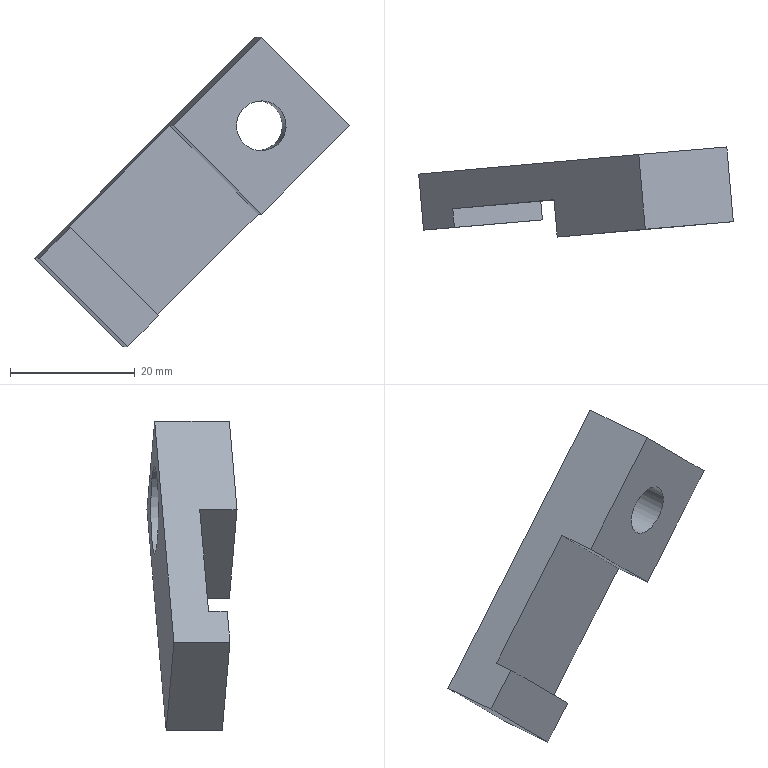Part | NX | features solid 2 | 1 solid | 13 faces | box 50.355 x 14.419 x 49.497 mm | volume 7701 mm3 | plane 11 | cylinder 1 | spline 1 | commonest cylinder face diameters 14 x1
STEP:
#1=CARTESIAN_POINT('',(-431.743,30.487,53.445));
#2=VERTEX_POINT('',#1);
#3=CARTESIAN_POINT('',(-415.541,31.905,69.708));
#4=VERTEX_POINT('',#3);
#5=CARTESIAN_POINT('',(-431.743,30.487,53.445));
#6=DIRECTION('',(0.7044,0.06163,0.7071));
#7=VECTOR('',#6,1000.);
#8=LINE('',#5,#7);
#9=EDGE_CURVE('',#2,#4,#8,.T.);
#10=ORIENTED_EDGE('',*,*,#9,.T.);
#11=CARTESIAN_POINT('',(-429.629,30.672,83.85));
#12=VERTEX_POINT('',#11);
#13=CARTESIAN_POINT('',(-415.541,31.905,69.708));
#14=DIRECTION('',(-0.7044,-0.06163,0.7071));
#15=VECTOR('',#14,1000.);
#16=LINE('',#13,#15);
#17=EDGE_CURVE('',#4,#12,#16,.T.);
#18=ORIENTED_EDGE('',*,*,#17,.T.);
#19=CARTESIAN_POINT('',(-445.831,29.255,67.587));
#20=VERTEX_POINT('',#19);
#21=CARTESIAN_POINT('',(-445.831,29.255,67.587));
#22=DIRECTION('',(0.7044,0.06163,0.7071));
#23=VECTOR('',#22,1000.);
#24=LINE('',#21,#23);
#25=EDGE_CURVE('',#20,#12,#24,.T.);
#26=ORIENTED_EDGE('',*,*,#25,.F.);
#27=CARTESIAN_POINT('',(-445.831,29.255,67.587));
#28=DIRECTION('',(0.7044,0.06163,-0.7071));
#29=VECTOR('',#28,1000.);
#30=LINE('',#27,#29);
#31=EDGE_CURVE('',#20,#2,#30,.T.);
#32=ORIENTED_EDGE('',*,*,#31,.T.);
#33=EDGE_LOOP('',(#10,#18,#26,#32));
#34=FACE_BOUND('',#33,.T.);
#35=CARTESIAN_POINT('',(-445.831,29.255,67.587));
#36=DIRECTION('',(-0.08716,0.9962,0.));
#37=DIRECTION('',(0.421,0.03683,0.9063));
#38=AXIS2_PLACEMENT_3D('',#35,#36,#37);
#39=PLANE('',#38);
#40=ADVANCED_FACE('',(#34),#39,.F.);
#41=CARTESIAN_POINT('',(-419.24,32.585,85.541));
#42=VERTEX_POINT('',#41);
#43=CARTESIAN_POINT('',(-420.152,32.505,83.576));
#44=CARTESIAN_POINT('',(-418.327,32.665,87.506));
#45=CARTESIAN_POINT('',(-415.894,32.878,88.387));
#46=CARTESIAN_POINT('',(-411.999,33.218,86.567));
#47=CARTESIAN_POINT('',(-411.109,33.296,84.118));
#48=CARTESIAN_POINT('',(-412.923,33.138,80.207));
#49=CARTESIAN_POINT('',(-415.352,32.925,79.311));
#50=CARTESIAN_POINT('',(-419.263,32.583,81.135));
#51=CARTESIAN_POINT('',(-420.152,32.505,83.576));
#52=CARTESIAN_POINT('',(-418.327,32.665,87.506));
#53=B_SPLINE_CURVE_WITH_KNOTS('',3,(#43,#44,#45,#46,#47,#48,#49,#50,#51,#52),.UNSPECIFIED.,.T.,.F.,(2,2,2,2,2,2,2),(-0.25,0.,0.25,0.5,0.75,1.,1.25),.UNSPECIFIED.);
#54=EDGE_CURVE('',#42,#42,#53,.T.);
#55=ORIENTED_EDGE('',*,*,#54,.F.);
#56=EDGE_LOOP('',(#55));
#57=FACE_BOUND('',#56,.T.);
#58=CARTESIAN_POINT('',(-419.115,32.596,77.788));
#59=VERTEX_POINT('',#58);
#60=CARTESIAN_POINT('',(-415.628,32.901,83.85));
#61=DIRECTION('',(0.08716,-0.9962,0.));
#62=DIRECTION('',(-0.4981,-0.04358,-0.866));
#63=AXIS2_PLACEMENT_3D('',#60,#61,#62);
#64=CIRCLE('',#63,7.);
#65=EDGE_CURVE('',#59,#59,#64,.T.);
#66=ORIENTED_EDGE('',*,*,#65,.F.);
#67=EDGE_LOOP('',(#66));
#68=FACE_BOUND('',#67,.T.);
#69=CARTESIAN_POINT('',(-415.628,32.901,83.85));
#70=DIRECTION('',(0.08716,-0.9962,0.));
#71=DIRECTION('',(0.9029,0.07899,-0.4226));
#72=AXIS2_PLACEMENT_3D('',#69,#70,#71);
#73=PLANE('',#72);
#74=ADVANCED_FACE('',(#57,#68),#73,.F.);
#75=CARTESIAN_POINT('',(-401.976,39.114,83.85));
#76=VERTEX_POINT('',#75);
#77=CARTESIAN_POINT('',(-437.196,36.033,48.495));
#78=VERTEX_POINT('',#77);
#79=CARTESIAN_POINT('',(-401.976,39.114,83.85));
#80=DIRECTION('',(-0.7044,-0.06163,-0.7071));
#81=VECTOR('',#80,1000.);
#82=LINE('',#79,#81);
#83=EDGE_CURVE('',#76,#78,#82,.T.);
#84=ORIENTED_EDGE('',*,*,#83,.T.);
#85=CARTESIAN_POINT('',(-451.285,34.8,62.637));
#86=VERTEX_POINT('',#85);
#87=CARTESIAN_POINT('',(-451.285,34.8,62.637));
#88=DIRECTION('',(0.7044,0.06163,-0.7071));
#89=VECTOR('',#88,1000.);
#90=LINE('',#87,#89);
#91=EDGE_CURVE('',#86,#78,#90,.T.);
#92=ORIENTED_EDGE('',*,*,#91,.F.);
#93=CARTESIAN_POINT('',(-416.064,37.882,97.992));
#94=VERTEX_POINT('',#93);
#95=CARTESIAN_POINT('',(-416.064,37.882,97.992));
#96=DIRECTION('',(-0.7044,-0.06163,-0.7071));
#97=VECTOR('',#96,1000.);
#98=LINE('',#95,#97);
#99=EDGE_CURVE('',#94,#86,#98,.T.);
#100=ORIENTED_EDGE('',*,*,#99,.F.);
#101=CARTESIAN_POINT('',(-416.064,37.882,97.992));
#102=DIRECTION('',(0.7044,0.06163,-0.7071));
#103=VECTOR('',#102,1000.);
#104=LINE('',#101,#103);
#105=EDGE_CURVE('',#94,#76,#104,.T.);
#106=ORIENTED_EDGE('',*,*,#105,.T.);
#107=EDGE_LOOP('',(#84,#92,#100,#106));
#108=FACE_BOUND('',#107,.T.);
#109=CARTESIAN_POINT('',(-409.744,38.435,80.892));
#110=VERTEX_POINT('',#109);
#111=CARTESIAN_POINT('',(-416.064,37.882,83.85));
#112=DIRECTION('',(0.08716,-0.9962,0.));
#113=DIRECTION('',(0.9029,0.07899,-0.4226));
#114=AXIS2_PLACEMENT_3D('',#111,#112,#113);
#115=CIRCLE('',#114,7.);
#116=EDGE_CURVE('',#110,#110,#115,.T.);
#117=ORIENTED_EDGE('',*,*,#116,.T.);
#118=EDGE_LOOP('',(#117));
#119=FACE_BOUND('',#118,.T.);
#120=CARTESIAN_POINT('',(-416.064,37.882,97.992));
#121=DIRECTION('',(0.08716,-0.9962,0.));
#122=DIRECTION('',(-0.421,-0.03683,-0.9063));
#123=AXIS2_PLACEMENT_3D('',#120,#121,#122);
#124=PLANE('',#123);
#125=ADVANCED_FACE('',(#108,#119),#124,.F.);
#126=CARTESIAN_POINT('',(-400.93,27.16,83.85));
#127=VERTEX_POINT('',#126);
#128=CARTESIAN_POINT('',(-401.976,39.114,83.85));
#129=DIRECTION('',(0.08716,-0.9962,0.));
#130=VECTOR('',#129,1000.);
#131=LINE('',#128,#130);
#132=EDGE_CURVE('',#76,#127,#131,.T.);
#133=ORIENTED_EDGE('',*,*,#132,.F.);
#134=ORIENTED_EDGE('',*,*,#105,.F.);
#135=CARTESIAN_POINT('',(-415.018,25.927,97.992));
#136=VERTEX_POINT('',#135);
#137=CARTESIAN_POINT('',(-416.064,37.882,97.992));
#138=DIRECTION('',(0.08716,-0.9962,0.));
#139=VECTOR('',#138,1000.);
#140=LINE('',#137,#139);
#141=EDGE_CURVE('',#94,#136,#140,.T.);
#142=ORIENTED_EDGE('',*,*,#141,.T.);
#143=CARTESIAN_POINT('',(-400.93,27.16,83.85));
#144=DIRECTION('',(-0.7044,-0.06163,0.7071));
#145=VECTOR('',#144,1000.);
#146=LINE('',#143,#145);
#147=EDGE_CURVE('',#127,#136,#146,.T.);
#148=ORIENTED_EDGE('',*,*,#147,.F.);
#149=EDGE_LOOP('',(#133,#134,#142,#148));
#150=FACE_BOUND('',#149,.T.);
#151=CARTESIAN_POINT('',(-416.064,37.882,97.992));
#152=DIRECTION('',(0.7044,0.06163,0.7071));
#153=DIRECTION('',(-0.7044,-0.06163,0.7071));
#154=AXIS2_PLACEMENT_3D('',#151,#152,#153);
#155=PLANE('',#154);
#156=ADVANCED_FACE('',(#150),#155,.T.);
#157=CARTESIAN_POINT('',(-436.412,27.067,48.495));
#158=VERTEX_POINT('',#157);
#159=CARTESIAN_POINT('',(-437.196,36.033,48.495));
#160=DIRECTION('',(0.08716,-0.9962,0.));
#161=VECTOR('',#160,1000.);
#162=LINE('',#159,#161);
#163=EDGE_CURVE('',#78,#158,#162,.T.);
#164=ORIENTED_EDGE('',*,*,#163,.T.);
#165=CARTESIAN_POINT('',(-450.5,25.835,62.637));
#166=VERTEX_POINT('',#165);
#167=CARTESIAN_POINT('',(-450.5,25.835,62.637));
#168=DIRECTION('',(0.7044,0.06163,-0.7071));
#169=VECTOR('',#168,1000.);
#170=LINE('',#167,#169);
#171=EDGE_CURVE('',#166,#158,#170,.T.);
#172=ORIENTED_EDGE('',*,*,#171,.F.);
#173=CARTESIAN_POINT('',(-451.285,34.8,62.637));
#174=DIRECTION('',(0.08716,-0.9962,0.));
#175=VECTOR('',#174,1000.);
#176=LINE('',#173,#175);
#177=EDGE_CURVE('',#86,#166,#176,.T.);
#178=ORIENTED_EDGE('',*,*,#177,.F.);
#179=ORIENTED_EDGE('',*,*,#91,.T.);
#180=EDGE_LOOP('',(#164,#172,#178,#179));
#181=FACE_BOUND('',#180,.T.);
#182=CARTESIAN_POINT('',(-451.285,34.8,62.637));
#183=DIRECTION('',(0.7044,0.06163,0.7071));
#184=DIRECTION('',(-0.7044,-0.06163,0.7071));
#185=AXIS2_PLACEMENT_3D('',#182,#183,#184);
#186=PLANE('',#185);
#187=ADVANCED_FACE('',(#181),#186,.F.);
#188=CARTESIAN_POINT('',(-431.481,27.499,53.445));
#189=VERTEX_POINT('',#188);
#190=CARTESIAN_POINT('',(-401.191,30.149,83.85));
#191=DIRECTION('',(-0.7044,-0.06163,-0.7071));
#192=VECTOR('',#191,1000.);
#193=LINE('',#190,#192);
#194=EDGE_CURVE('',#189,#158,#193,.T.);
#195=ORIENTED_EDGE('',*,*,#194,.F.);
#196=CARTESIAN_POINT('',(-445.569,26.266,67.587));
#197=VERTEX_POINT('',#196);
#198=CARTESIAN_POINT('',(-445.569,26.266,67.587));
#199=DIRECTION('',(0.7044,0.06163,-0.7071));
#200=VECTOR('',#199,1000.);
#201=LINE('',#198,#200);
#202=EDGE_CURVE('',#197,#189,#201,.T.);
#203=ORIENTED_EDGE('',*,*,#202,.F.);
#204=CARTESIAN_POINT('',(-415.279,28.916,97.992));
#205=DIRECTION('',(-0.7044,-0.06163,-0.7071));
#206=VECTOR('',#205,1000.);
#207=LINE('',#204,#206);
#208=EDGE_CURVE('',#197,#166,#207,.T.);
#209=ORIENTED_EDGE('',*,*,#208,.T.);
#210=ORIENTED_EDGE('',*,*,#171,.T.);
#211=EDGE_LOOP('',(#195,#203,#209,#210));
#212=FACE_BOUND('',#211,.T.);
#213=CARTESIAN_POINT('',(-445.569,26.266,67.587));
#214=DIRECTION('',(0.08716,-0.9962,0.));
#215=DIRECTION('',(-0.421,-0.03683,-0.9063));
#216=AXIS2_PLACEMENT_3D('',#213,#214,#215);
#217=PLANE('',#216);
#218=ADVANCED_FACE('',(#212),#217,.T.);
#219=CARTESIAN_POINT('',(-431.743,30.487,53.445));
#220=DIRECTION('',(0.08716,-0.9962,0.));
#221=VECTOR('',#220,1000.);
#222=LINE('',#219,#221);
#223=EDGE_CURVE('',#2,#189,#222,.T.);
#224=ORIENTED_EDGE('',*,*,#223,.F.);
#225=ORIENTED_EDGE('',*,*,#31,.F.);
#226=CARTESIAN_POINT('',(-445.744,28.258,67.587));
#227=DIRECTION('',(0.08716,-0.9962,0.));
#228=VECTOR('',#227,1000.);
#229=LINE('',#226,#228);
#230=EDGE_CURVE('',#20,#197,#229,.T.);
#231=ORIENTED_EDGE('',*,*,#230,.T.);
#232=ORIENTED_EDGE('',*,*,#202,.T.);
#233=EDGE_LOOP('',(#224,#225,#231,#232));
#234=FACE_BOUND('',#233,.T.);
#235=CARTESIAN_POINT('',(-445.831,29.255,67.587));
#236=DIRECTION('',(0.7044,0.06163,0.7071));
#237=DIRECTION('',(-0.7044,-0.06163,0.7071));
#238=AXIS2_PLACEMENT_3D('',#235,#236,#237);
#239=PLANE('',#238);
#240=ADVANCED_FACE('',(#234),#239,.T.);
#241=ORIENTED_EDGE('',*,*,#25,.T.);
#242=CARTESIAN_POINT('',(-429.106,24.695,83.85));
#243=VERTEX_POINT('',#242);
#244=CARTESIAN_POINT('',(-429.106,24.695,83.85));
#245=DIRECTION('',(-0.08716,0.9962,0.));
#246=VECTOR('',#245,1000.);
#247=LINE('',#244,#246);
#248=EDGE_CURVE('',#243,#12,#247,.T.);
#249=ORIENTED_EDGE('',*,*,#248,.F.);
#250=CARTESIAN_POINT('',(-415.018,25.927,97.992));
#251=DIRECTION('',(-0.7044,-0.06163,-0.7071));
#252=VECTOR('',#251,1000.);
#253=LINE('',#250,#252);
#254=EDGE_CURVE('',#136,#243,#253,.T.);
#255=ORIENTED_EDGE('',*,*,#254,.F.);
#256=ORIENTED_EDGE('',*,*,#141,.F.);
#257=ORIENTED_EDGE('',*,*,#99,.T.);
#258=ORIENTED_EDGE('',*,*,#177,.T.);
#259=ORIENTED_EDGE('',*,*,#208,.F.);
#260=ORIENTED_EDGE('',*,*,#230,.F.);
#261=EDGE_LOOP('',(#241,#249,#255,#256,#257,#258,#259,#260));
#262=FACE_BOUND('',#261,.T.);
#263=CARTESIAN_POINT('',(-415.541,31.905,97.992));
#264=DIRECTION('',(0.7044,0.06163,-0.7071));
#265=DIRECTION('',(0.7044,0.06163,0.7071));
#266=AXIS2_PLACEMENT_3D('',#263,#264,#265);
#267=PLANE('',#266);
#268=ADVANCED_FACE('',(#262),#267,.F.);
#269=ORIENTED_EDGE('',*,*,#9,.F.);
#270=ORIENTED_EDGE('',*,*,#223,.T.);
#271=ORIENTED_EDGE('',*,*,#194,.T.);
#272=ORIENTED_EDGE('',*,*,#163,.F.);
#273=ORIENTED_EDGE('',*,*,#83,.F.);
#274=ORIENTED_EDGE('',*,*,#132,.T.);
#275=CARTESIAN_POINT('',(-415.018,25.927,69.708));
#276=VERTEX_POINT('',#275);
#277=CARTESIAN_POINT('',(-400.93,27.16,83.85));
#278=DIRECTION('',(-0.7044,-0.06163,-0.7071));
#279=VECTOR('',#278,1000.);
#280=LINE('',#277,#279);
#281=EDGE_CURVE('',#127,#276,#280,.T.);
#282=ORIENTED_EDGE('',*,*,#281,.T.);
#283=CARTESIAN_POINT('',(-415.018,25.927,69.708));
#284=DIRECTION('',(-0.08716,0.9962,0.));
#285=VECTOR('',#284,1000.);
#286=LINE('',#283,#285);
#287=EDGE_CURVE('',#276,#4,#286,.T.);
#288=ORIENTED_EDGE('',*,*,#287,.T.);
#289=EDGE_LOOP('',(#269,#270,#271,#272,#273,#274,#282,#288));
#290=FACE_BOUND('',#289,.T.);
#291=CARTESIAN_POINT('',(-401.453,33.137,83.85));
#292=DIRECTION('',(0.7044,0.06163,-0.7071));
#293=DIRECTION('',(0.7044,0.06163,0.7071));
#294=AXIS2_PLACEMENT_3D('',#291,#292,#293);
#295=PLANE('',#294);
#296=ADVANCED_FACE('',(#290),#295,.T.);
#297=ORIENTED_EDGE('',*,*,#65,.T.);
#298=EDGE_LOOP('',(#297));
#299=FACE_BOUND('',#298,.T.);
#300=ORIENTED_EDGE('',*,*,#116,.F.);
#301=EDGE_LOOP('',(#300));
#302=FACE_BOUND('',#301,.T.);
#303=CARTESIAN_POINT('',(-415.802,34.893,83.85));
#304=DIRECTION('',(-0.08716,0.9962,0.));
#305=DIRECTION('',(-0.9029,-0.07899,0.4226));
#306=AXIS2_PLACEMENT_3D('',#303,#304,#305);
#307=CYLINDRICAL_SURFACE('',#306,7.);
#308=ADVANCED_FACE('',(#299,#302),#307,.F.);
#309=ORIENTED_EDGE('',*,*,#17,.F.);
#310=ORIENTED_EDGE('',*,*,#287,.F.);
#311=CARTESIAN_POINT('',(-415.018,25.927,69.708));
#312=DIRECTION('',(-0.7044,-0.06163,0.7071));
#313=VECTOR('',#312,1000.);
#314=LINE('',#311,#313);
#315=EDGE_CURVE('',#276,#243,#314,.T.);
#316=ORIENTED_EDGE('',*,*,#315,.T.);
#317=ORIENTED_EDGE('',*,*,#248,.T.);
#318=EDGE_LOOP('',(#309,#310,#316,#317));
#319=FACE_BOUND('',#318,.T.);
#320=CARTESIAN_POINT('',(-415.018,25.927,69.708));
#321=DIRECTION('',(-0.7044,-0.06163,-0.7071));
#322=DIRECTION('',(-0.7044,-0.06163,0.7071));
#323=AXIS2_PLACEMENT_3D('',#320,#321,#322);
#324=PLANE('',#323);
#325=ADVANCED_FACE('',(#319),#324,.T.);
#326=CARTESIAN_POINT('',(-418.629,25.611,85.541));
#327=VERTEX_POINT('',#326);
#328=CARTESIAN_POINT('',(-419.542,25.532,83.576));
#329=CARTESIAN_POINT('',(-417.717,25.691,87.506));
#330=CARTESIAN_POINT('',(-415.284,25.904,88.387));
#331=CARTESIAN_POINT('',(-411.389,26.245,86.567));
#332=CARTESIAN_POINT('',(-410.499,26.323,84.118));
#333=CARTESIAN_POINT('',(-412.312,26.164,80.207));
#334=CARTESIAN_POINT('',(-414.742,25.952,79.311));
#335=CARTESIAN_POINT('',(-418.653,25.609,81.135));
#336=CARTESIAN_POINT('',(-419.542,25.532,83.576));
#337=CARTESIAN_POINT('',(-417.717,25.691,87.506));
#338=B_SPLINE_CURVE_WITH_KNOTS('',3,(#328,#329,#330,#331,#332,#333,#334,#335,#336,#337),.UNSPECIFIED.,.T.,.F.,(2,2,2,2,2,2,2),(-0.25,0.,0.25,0.5,0.75,1.,1.25),.UNSPECIFIED.);
#339=EDGE_CURVE('',#327,#327,#338,.T.);
#340=ORIENTED_EDGE('',*,*,#339,.T.);
#341=EDGE_LOOP('',(#340));
#342=FACE_BOUND('',#341,.T.);
#343=ORIENTED_EDGE('',*,*,#281,.F.);
#344=ORIENTED_EDGE('',*,*,#147,.T.);
#345=ORIENTED_EDGE('',*,*,#254,.T.);
#346=ORIENTED_EDGE('',*,*,#315,.F.);
#347=EDGE_LOOP('',(#343,#344,#345,#346));
#348=FACE_BOUND('',#347,.T.);
#349=CARTESIAN_POINT('',(-415.018,25.927,69.708));
#350=DIRECTION('',(-0.08716,0.9962,0.));
#351=DIRECTION('',(0.4981,0.04358,0.866));
#352=AXIS2_PLACEMENT_3D('',#349,#350,#351);
#353=PLANE('',#352);
#354=ADVANCED_FACE('',(#342,#348),#353,.F.);
#355=ORIENTED_EDGE('',*,*,#54,.T.);
#356=EDGE_LOOP('',(#355));
#357=FACE_BOUND('',#356,.T.);
#358=ORIENTED_EDGE('',*,*,#339,.F.);
#359=EDGE_LOOP('',(#358));
#360=FACE_BOUND('',#359,.T.);
#361=CARTESIAN_POINT('',(-419.129,25.568,82.344));
#362=CARTESIAN_POINT('',(-419.739,32.541,82.344));
#363=CARTESIAN_POINT('',(-419.034,25.576,85.731));
#364=CARTESIAN_POINT('',(-419.644,32.549,85.731));
#365=CARTESIAN_POINT('',(-416.511,25.797,87.977));
#366=CARTESIAN_POINT('',(-417.121,32.77,87.977));
#367=CARTESIAN_POINT('',(-413.149,26.091,87.883));
#368=CARTESIAN_POINT('',(-413.759,33.064,87.883));
#369=CARTESIAN_POINT('',(-410.914,26.287,85.354));
#370=CARTESIAN_POINT('',(-411.524,33.26,85.354));
#371=CARTESIAN_POINT('',(-411.001,26.279,81.973));
#372=CARTESIAN_POINT('',(-411.611,33.252,81.973));
#373=CARTESIAN_POINT('',(-413.516,26.059,79.728));
#374=CARTESIAN_POINT('',(-414.126,33.032,79.728));
#375=CARTESIAN_POINT('',(-416.885,25.764,79.816));
#376=CARTESIAN_POINT('',(-417.495,32.737,79.816));
#377=CARTESIAN_POINT('',(-419.129,25.568,82.344));
#378=CARTESIAN_POINT('',(-419.739,32.541,82.344));
#379=CARTESIAN_POINT('',(-419.034,25.576,85.731));
#380=CARTESIAN_POINT('',(-419.644,32.549,85.731));
#381=CARTESIAN_POINT('',(-416.511,25.797,87.977));
#382=CARTESIAN_POINT('',(-417.121,32.77,87.977));
#383=B_SPLINE_SURFACE_WITH_KNOTS('',3,1,((#361,#362),(#363,#364),(#365,#366),(#367,#368),(#369,#370),(#371,#372),(#373,#374),(#375,#376),(#377,#378),(#379,#380),(#381,#382)),.SURF_OF_LINEAR_EXTRUSION.,.T.,.F.,.F.,(1,1,1,1,1,1,1,1,1,1,1,1,1,1,1),(2,2),(-0.375,-0.25,-0.125,0.,0.125,0.25,0.375,0.5,0.625,0.75,0.875,1.,1.125,1.25,1.375),(0.,1.),.UNSPECIFIED.);
#384=ADVANCED_FACE('',(#357,#360),#383,.F.);
#385=CLOSED_SHELL('',(#40,#74,#125,#156,#187,#218,#240,#268,#296,#308,#325,#354,#384));
#386=MANIFOLD_SOLID_BREP('',#385);
#387=(LENGTH_UNIT()NAMED_UNIT(*)SI_UNIT(.MILLI.,.METRE.));
#388=UNCERTAINTY_MEASURE_WITH_UNIT(LENGTH_MEASURE(0.0508),#387,'','');
#389=(NAMED_UNIT(*)PLANE_ANGLE_UNIT()SI_UNIT($,.RADIAN.));
#390=(NAMED_UNIT(*)SI_UNIT($,.STERADIAN.)SOLID_ANGLE_UNIT());
#391=(GEOMETRIC_REPRESENTATION_CONTEXT(3)GLOBAL_UNCERTAINTY_ASSIGNED_CONTEXT((#388))GLOBAL_UNIT_ASSIGNED_CONTEXT((#387,#389,#390))REPRESENTATION_CONTEXT('',''));
#392=ADVANCED_BREP_SHAPE_REPRESENTATION('',(#386),#391);